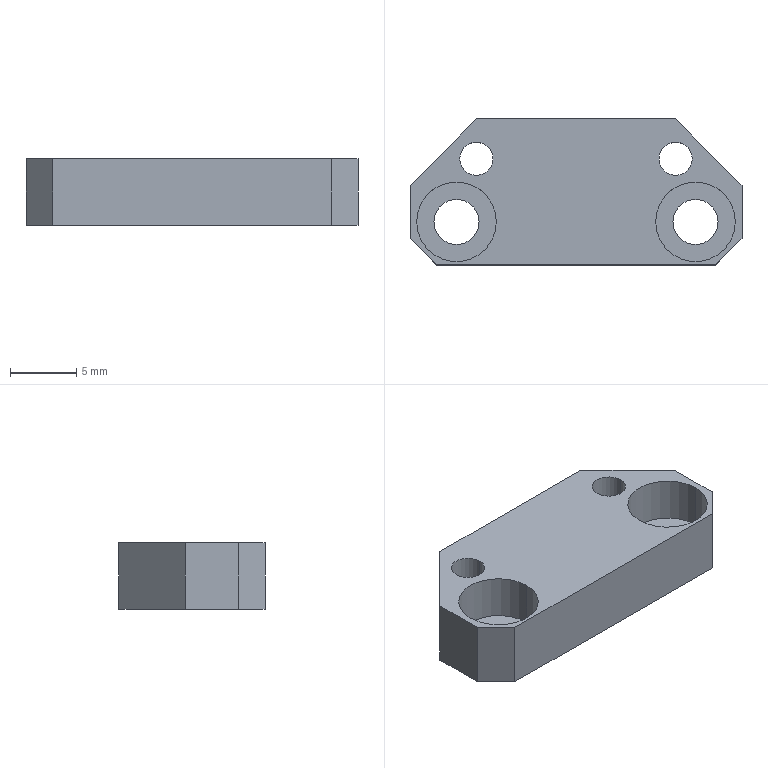Part | SolidWorks | features Chamfer 2, HoleWzd 2, Extrusion 1 | 1 solid | 24 faces | box 25 x 11 x 5 mm | volume 959.594 mm3 | cylinder 12 | plane 12 | commonest cylinder face diameters 2.5 x4 3.4 x4 6 x4
STEP:
#1=CARTESIAN_POINT('',(6.,-2.25,-0.9));
#2=VERTEX_POINT('',#1);
#3=CARTESIAN_POINT('',(12.,-2.25,-0.9));
#4=VERTEX_POINT('',#3);
#5=CARTESIAN_POINT('',(9.,-2.25,-0.9));
#6=DIRECTION('',(0.,0.,1.));
#7=DIRECTION('',(1.,0.,0.));
#8=AXIS2_PLACEMENT_3D('',#5,#6,#7);
#9=CIRCLE('',#8,3.);
#10=EDGE_CURVE('',#2,#4,#9,.T.);
#11=ORIENTED_EDGE('',*,*,#10,.F.);
#12=CARTESIAN_POINT('',(6.,-2.25,2.5));
#13=VERTEX_POINT('',#12);
#14=CARTESIAN_POINT('',(6.,-2.25,2.5));
#15=DIRECTION('',(0.,0.,1.));
#16=VECTOR('',#15,1000.);
#17=LINE('',#14,#16);
#18=EDGE_CURVE('',#2,#13,#17,.T.);
#19=ORIENTED_EDGE('',*,*,#18,.T.);
#20=CARTESIAN_POINT('',(12.,-2.25,2.5));
#21=VERTEX_POINT('',#20);
#22=CARTESIAN_POINT('',(9.,-2.25,2.5));
#23=DIRECTION('',(0.,0.,1.));
#24=DIRECTION('',(1.,0.,0.));
#25=AXIS2_PLACEMENT_3D('',#22,#23,#24);
#26=CIRCLE('',#25,3.);
#27=EDGE_CURVE('',#13,#21,#26,.T.);
#28=ORIENTED_EDGE('',*,*,#27,.T.);
#29=CARTESIAN_POINT('',(12.,-2.25,2.5));
#30=DIRECTION('',(0.,0.,1.));
#31=VECTOR('',#30,1000.);
#32=LINE('',#29,#31);
#33=EDGE_CURVE('',#4,#21,#32,.T.);
#34=ORIENTED_EDGE('',*,*,#33,.F.);
#35=EDGE_LOOP('',(#11,#19,#28,#34));
#36=FACE_OUTER_BOUND('',#35,.T.);
#37=CARTESIAN_POINT('',(9.,-2.25,2.5));
#38=DIRECTION('',(0.,0.,1.));
#39=DIRECTION('',(1.,0.,0.));
#40=AXIS2_PLACEMENT_3D('',#37,#38,#39);
#41=CYLINDRICAL_SURFACE('',#40,3.);
#42=ADVANCED_FACE('',(#36),#41,.F.);
#43=CARTESIAN_POINT('',(7.3,-2.25,-2.5));
#44=VERTEX_POINT('',#43);
#45=CARTESIAN_POINT('',(10.7,-2.25,-2.5));
#46=VERTEX_POINT('',#45);
#47=CARTESIAN_POINT('',(9.,-2.25,-2.5));
#48=DIRECTION('',(0.,0.,1.));
#49=DIRECTION('',(1.,0.,0.));
#50=AXIS2_PLACEMENT_3D('',#47,#48,#49);
#51=CIRCLE('',#50,1.7);
#52=EDGE_CURVE('',#44,#46,#51,.T.);
#53=ORIENTED_EDGE('',*,*,#52,.F.);
#54=CARTESIAN_POINT('',(7.3,-2.25,-0.9));
#55=VERTEX_POINT('',#54);
#56=CARTESIAN_POINT('',(7.3,-2.25,2.5));
#57=DIRECTION('',(0.,0.,1.));
#58=VECTOR('',#57,1000.);
#59=LINE('',#56,#58);
#60=EDGE_CURVE('',#44,#55,#59,.T.);
#61=ORIENTED_EDGE('',*,*,#60,.T.);
#62=CARTESIAN_POINT('',(10.7,-2.25,-0.9));
#63=VERTEX_POINT('',#62);
#64=CARTESIAN_POINT('',(9.,-2.25,-0.9));
#65=DIRECTION('',(0.,0.,1.));
#66=DIRECTION('',(1.,0.,0.));
#67=AXIS2_PLACEMENT_3D('',#64,#65,#66);
#68=CIRCLE('',#67,1.7);
#69=EDGE_CURVE('',#55,#63,#68,.T.);
#70=ORIENTED_EDGE('',*,*,#69,.T.);
#71=CARTESIAN_POINT('',(10.7,-2.25,2.5));
#72=DIRECTION('',(0.,0.,1.));
#73=VECTOR('',#72,1000.);
#74=LINE('',#71,#73);
#75=EDGE_CURVE('',#46,#63,#74,.T.);
#76=ORIENTED_EDGE('',*,*,#75,.F.);
#77=EDGE_LOOP('',(#53,#61,#70,#76));
#78=FACE_OUTER_BOUND('',#77,.T.);
#79=CARTESIAN_POINT('',(9.,-2.25,2.5));
#80=DIRECTION('',(0.,0.,1.));
#81=DIRECTION('',(1.,0.,0.));
#82=AXIS2_PLACEMENT_3D('',#79,#80,#81);
#83=CYLINDRICAL_SURFACE('',#82,1.7);
#84=ADVANCED_FACE('',(#78),#83,.F.);
#85=CARTESIAN_POINT('',(-12.,-2.25,-0.9));
#86=VERTEX_POINT('',#85);
#87=CARTESIAN_POINT('',(-6.,-2.25,-0.9));
#88=VERTEX_POINT('',#87);
#89=CARTESIAN_POINT('',(-9.,-2.25,-0.9));
#90=DIRECTION('',(0.,0.,1.));
#91=DIRECTION('',(1.,0.,0.));
#92=AXIS2_PLACEMENT_3D('',#89,#90,#91);
#93=CIRCLE('',#92,3.);
#94=EDGE_CURVE('',#86,#88,#93,.T.);
#95=ORIENTED_EDGE('',*,*,#94,.F.);
#96=CARTESIAN_POINT('',(-12.,-2.25,2.5));
#97=VERTEX_POINT('',#96);
#98=CARTESIAN_POINT('',(-12.,-2.25,2.5));
#99=DIRECTION('',(0.,0.,1.));
#100=VECTOR('',#99,1000.);
#101=LINE('',#98,#100);
#102=EDGE_CURVE('',#86,#97,#101,.T.);
#103=ORIENTED_EDGE('',*,*,#102,.T.);
#104=CARTESIAN_POINT('',(-6.,-2.25,2.5));
#105=VERTEX_POINT('',#104);
#106=CARTESIAN_POINT('',(-9.,-2.25,2.5));
#107=DIRECTION('',(0.,0.,1.));
#108=DIRECTION('',(1.,0.,0.));
#109=AXIS2_PLACEMENT_3D('',#106,#107,#108);
#110=CIRCLE('',#109,3.);
#111=EDGE_CURVE('',#97,#105,#110,.T.);
#112=ORIENTED_EDGE('',*,*,#111,.T.);
#113=CARTESIAN_POINT('',(-6.,-2.25,2.5));
#114=DIRECTION('',(0.,0.,1.));
#115=VECTOR('',#114,1000.);
#116=LINE('',#113,#115);
#117=EDGE_CURVE('',#88,#105,#116,.T.);
#118=ORIENTED_EDGE('',*,*,#117,.F.);
#119=EDGE_LOOP('',(#95,#103,#112,#118));
#120=FACE_OUTER_BOUND('',#119,.T.);
#121=CARTESIAN_POINT('',(-9.,-2.25,2.5));
#122=DIRECTION('',(0.,0.,1.));
#123=DIRECTION('',(1.,0.,0.));
#124=AXIS2_PLACEMENT_3D('',#121,#122,#123);
#125=CYLINDRICAL_SURFACE('',#124,3.);
#126=ADVANCED_FACE('',(#120),#125,.F.);
#127=CARTESIAN_POINT('',(-10.7,-2.25,-2.5));
#128=VERTEX_POINT('',#127);
#129=CARTESIAN_POINT('',(-7.3,-2.25,-2.5));
#130=VERTEX_POINT('',#129);
#131=CARTESIAN_POINT('',(-9.,-2.25,-2.5));
#132=DIRECTION('',(0.,0.,1.));
#133=DIRECTION('',(1.,0.,0.));
#134=AXIS2_PLACEMENT_3D('',#131,#132,#133);
#135=CIRCLE('',#134,1.7);
#136=EDGE_CURVE('',#128,#130,#135,.T.);
#137=ORIENTED_EDGE('',*,*,#136,.F.);
#138=CARTESIAN_POINT('',(-10.7,-2.25,-0.9));
#139=VERTEX_POINT('',#138);
#140=CARTESIAN_POINT('',(-10.7,-2.25,2.5));
#141=DIRECTION('',(0.,0.,1.));
#142=VECTOR('',#141,1000.);
#143=LINE('',#140,#142);
#144=EDGE_CURVE('',#128,#139,#143,.T.);
#145=ORIENTED_EDGE('',*,*,#144,.T.);
#146=CARTESIAN_POINT('',(-7.3,-2.25,-0.9));
#147=VERTEX_POINT('',#146);
#148=CARTESIAN_POINT('',(-9.,-2.25,-0.9));
#149=DIRECTION('',(0.,0.,1.));
#150=DIRECTION('',(1.,0.,0.));
#151=AXIS2_PLACEMENT_3D('',#148,#149,#150);
#152=CIRCLE('',#151,1.7);
#153=EDGE_CURVE('',#139,#147,#152,.T.);
#154=ORIENTED_EDGE('',*,*,#153,.T.);
#155=CARTESIAN_POINT('',(-7.3,-2.25,2.5));
#156=DIRECTION('',(0.,0.,1.));
#157=VECTOR('',#156,1000.);
#158=LINE('',#155,#157);
#159=EDGE_CURVE('',#130,#147,#158,.T.);
#160=ORIENTED_EDGE('',*,*,#159,.F.);
#161=EDGE_LOOP('',(#137,#145,#154,#160));
#162=FACE_OUTER_BOUND('',#161,.T.);
#163=CARTESIAN_POINT('',(-9.,-2.25,2.5));
#164=DIRECTION('',(0.,0.,1.));
#165=DIRECTION('',(1.,0.,0.));
#166=AXIS2_PLACEMENT_3D('',#163,#164,#165);
#167=CYLINDRICAL_SURFACE('',#166,1.7);
#168=ADVANCED_FACE('',(#162),#167,.F.);
#169=CARTESIAN_POINT('',(-8.75,2.5,-2.5));
#170=VERTEX_POINT('',#169);
#171=CARTESIAN_POINT('',(-6.25,2.5,-2.5));
#172=VERTEX_POINT('',#171);
#173=CARTESIAN_POINT('',(-7.5,2.5,-2.5));
#174=DIRECTION('',(0.,0.,1.));
#175=DIRECTION('',(1.,0.,0.));
#176=AXIS2_PLACEMENT_3D('',#173,#174,#175);
#177=CIRCLE('',#176,1.25);
#178=EDGE_CURVE('',#170,#172,#177,.T.);
#179=ORIENTED_EDGE('',*,*,#178,.F.);
#180=CARTESIAN_POINT('',(-8.75,2.5,2.5));
#181=VERTEX_POINT('',#180);
#182=CARTESIAN_POINT('',(-8.75,2.5,2.5));
#183=DIRECTION('',(0.,0.,1.));
#184=VECTOR('',#183,1000.);
#185=LINE('',#182,#184);
#186=EDGE_CURVE('',#170,#181,#185,.T.);
#187=ORIENTED_EDGE('',*,*,#186,.T.);
#188=CARTESIAN_POINT('',(-6.25,2.5,2.5));
#189=VERTEX_POINT('',#188);
#190=CARTESIAN_POINT('',(-7.5,2.5,2.5));
#191=DIRECTION('',(0.,0.,1.));
#192=DIRECTION('',(1.,0.,0.));
#193=AXIS2_PLACEMENT_3D('',#190,#191,#192);
#194=CIRCLE('',#193,1.25);
#195=EDGE_CURVE('',#181,#189,#194,.T.);
#196=ORIENTED_EDGE('',*,*,#195,.T.);
#197=CARTESIAN_POINT('',(-6.25,2.5,2.5));
#198=DIRECTION('',(0.,0.,1.));
#199=VECTOR('',#198,1000.);
#200=LINE('',#197,#199);
#201=EDGE_CURVE('',#172,#189,#200,.T.);
#202=ORIENTED_EDGE('',*,*,#201,.F.);
#203=EDGE_LOOP('',(#179,#187,#196,#202));
#204=FACE_OUTER_BOUND('',#203,.T.);
#205=CARTESIAN_POINT('',(-7.5,2.5,2.5));
#206=DIRECTION('',(0.,0.,1.));
#207=DIRECTION('',(1.,0.,0.));
#208=AXIS2_PLACEMENT_3D('',#205,#206,#207);
#209=CYLINDRICAL_SURFACE('',#208,1.25);
#210=ADVANCED_FACE('',(#204),#209,.F.);
#211=CARTESIAN_POINT('',(6.25,2.5,-2.5));
#212=VERTEX_POINT('',#211);
#213=CARTESIAN_POINT('',(8.75,2.5,-2.5));
#214=VERTEX_POINT('',#213);
#215=CARTESIAN_POINT('',(7.5,2.5,-2.5));
#216=DIRECTION('',(0.,0.,1.));
#217=DIRECTION('',(1.,0.,0.));
#218=AXIS2_PLACEMENT_3D('',#215,#216,#217);
#219=CIRCLE('',#218,1.25);
#220=EDGE_CURVE('',#212,#214,#219,.T.);
#221=ORIENTED_EDGE('',*,*,#220,.F.);
#222=CARTESIAN_POINT('',(6.25,2.5,2.5));
#223=VERTEX_POINT('',#222);
#224=CARTESIAN_POINT('',(6.25,2.5,2.5));
#225=DIRECTION('',(0.,0.,1.));
#226=VECTOR('',#225,1000.);
#227=LINE('',#224,#226);
#228=EDGE_CURVE('',#212,#223,#227,.T.);
#229=ORIENTED_EDGE('',*,*,#228,.T.);
#230=CARTESIAN_POINT('',(8.75,2.5,2.5));
#231=VERTEX_POINT('',#230);
#232=CARTESIAN_POINT('',(7.5,2.5,2.5));
#233=DIRECTION('',(0.,0.,1.));
#234=DIRECTION('',(1.,0.,0.));
#235=AXIS2_PLACEMENT_3D('',#232,#233,#234);
#236=CIRCLE('',#235,1.25);
#237=EDGE_CURVE('',#223,#231,#236,.T.);
#238=ORIENTED_EDGE('',*,*,#237,.T.);
#239=CARTESIAN_POINT('',(8.75,2.5,2.5));
#240=DIRECTION('',(0.,0.,1.));
#241=VECTOR('',#240,1000.);
#242=LINE('',#239,#241);
#243=EDGE_CURVE('',#214,#231,#242,.T.);
#244=ORIENTED_EDGE('',*,*,#243,.F.);
#245=EDGE_LOOP('',(#221,#229,#238,#244));
#246=FACE_OUTER_BOUND('',#245,.T.);
#247=CARTESIAN_POINT('',(7.5,2.5,2.5));
#248=DIRECTION('',(0.,0.,1.));
#249=DIRECTION('',(1.,0.,0.));
#250=AXIS2_PLACEMENT_3D('',#247,#248,#249);
#251=CYLINDRICAL_SURFACE('',#250,1.25);
#252=ADVANCED_FACE('',(#246),#251,.F.);
#253=CARTESIAN_POINT('',(-7.5,5.5,-2.5));
#254=VERTEX_POINT('',#253);
#255=CARTESIAN_POINT('',(7.5,5.5,-2.5));
#256=VERTEX_POINT('',#255);
#257=CARTESIAN_POINT('',(0.,5.5,-2.5));
#258=DIRECTION('',(1.,0.,0.));
#259=VECTOR('',#258,1000.);
#260=LINE('',#257,#259);
#261=EDGE_CURVE('',#254,#256,#260,.T.);
#262=ORIENTED_EDGE('',*,*,#261,.F.);
#263=CARTESIAN_POINT('',(-7.5,5.5,2.5));
#264=VERTEX_POINT('',#263);
#265=CARTESIAN_POINT('',(-7.5,5.5,2.5));
#266=DIRECTION('',(0.,0.,1.));
#267=VECTOR('',#266,1000.);
#268=LINE('',#265,#267);
#269=EDGE_CURVE('',#254,#264,#268,.T.);
#270=ORIENTED_EDGE('',*,*,#269,.T.);
#271=CARTESIAN_POINT('',(7.5,5.5,2.5));
#272=VERTEX_POINT('',#271);
#273=CARTESIAN_POINT('',(0.,5.5,2.5));
#274=DIRECTION('',(1.,0.,0.));
#275=VECTOR('',#274,1000.);
#276=LINE('',#273,#275);
#277=EDGE_CURVE('',#264,#272,#276,.T.);
#278=ORIENTED_EDGE('',*,*,#277,.T.);
#279=CARTESIAN_POINT('',(7.5,5.5,-2.5));
#280=DIRECTION('',(0.,0.,-1.));
#281=VECTOR('',#280,1000.);
#282=LINE('',#279,#281);
#283=EDGE_CURVE('',#272,#256,#282,.T.);
#284=ORIENTED_EDGE('',*,*,#283,.T.);
#285=EDGE_LOOP('',(#262,#270,#278,#284));
#286=FACE_OUTER_BOUND('',#285,.T.);
#287=CARTESIAN_POINT('',(0.,5.5,2.5));
#288=DIRECTION('',(0.,1.,0.));
#289=DIRECTION('',(0.,0.,1.));
#290=AXIS2_PLACEMENT_3D('',#287,#288,#289);
#291=PLANE('',#290);
#292=ADVANCED_FACE('',(#286),#291,.T.);
#293=CARTESIAN_POINT('',(-12.5,-3.5,-2.5));
#294=VERTEX_POINT('',#293);
#295=CARTESIAN_POINT('',(-12.5,0.5,-2.5));
#296=VERTEX_POINT('',#295);
#297=CARTESIAN_POINT('',(-12.5,0.,-2.5));
#298=DIRECTION('',(0.,1.,0.));
#299=VECTOR('',#298,1000.);
#300=LINE('',#297,#299);
#301=EDGE_CURVE('',#294,#296,#300,.T.);
#302=ORIENTED_EDGE('',*,*,#301,.F.);
#303=CARTESIAN_POINT('',(-12.5,-3.5,2.5));
#304=VERTEX_POINT('',#303);
#305=CARTESIAN_POINT('',(-12.5,-3.5,2.5));
#306=DIRECTION('',(0.,0.,1.));
#307=VECTOR('',#306,1000.);
#308=LINE('',#305,#307);
#309=EDGE_CURVE('',#294,#304,#308,.T.);
#310=ORIENTED_EDGE('',*,*,#309,.T.);
#311=CARTESIAN_POINT('',(-12.5,0.5,2.5));
#312=VERTEX_POINT('',#311);
#313=CARTESIAN_POINT('',(-12.5,0.,2.5));
#314=DIRECTION('',(0.,1.,0.));
#315=VECTOR('',#314,1000.);
#316=LINE('',#313,#315);
#317=EDGE_CURVE('',#304,#312,#316,.T.);
#318=ORIENTED_EDGE('',*,*,#317,.T.);
#319=CARTESIAN_POINT('',(-12.5,0.5,2.5));
#320=DIRECTION('',(0.,0.,-1.));
#321=VECTOR('',#320,1000.);
#322=LINE('',#319,#321);
#323=EDGE_CURVE('',#312,#296,#322,.T.);
#324=ORIENTED_EDGE('',*,*,#323,.T.);
#325=EDGE_LOOP('',(#302,#310,#318,#324));
#326=FACE_OUTER_BOUND('',#325,.T.);
#327=CARTESIAN_POINT('',(-12.5,0.,2.5));
#328=DIRECTION('',(-1.,0.,0.));
#329=DIRECTION('',(0.,0.,1.));
#330=AXIS2_PLACEMENT_3D('',#327,#328,#329);
#331=PLANE('',#330);
#332=ADVANCED_FACE('',(#326),#331,.T.);
#333=CARTESIAN_POINT('',(-10.5,-5.5,2.5));
#334=VERTEX_POINT('',#333);
#335=CARTESIAN_POINT('',(10.5,-5.5,2.5));
#336=VERTEX_POINT('',#335);
#337=CARTESIAN_POINT('',(0.,-5.5,2.5));
#338=DIRECTION('',(1.,0.,0.));
#339=VECTOR('',#338,1000.);
#340=LINE('',#337,#339);
#341=EDGE_CURVE('',#334,#336,#340,.T.);
#342=ORIENTED_EDGE('',*,*,#341,.F.);
#343=CARTESIAN_POINT('',(-10.5,-5.5,-2.5));
#344=VERTEX_POINT('',#343);
#345=CARTESIAN_POINT('',(-10.5,-5.5,-2.5));
#346=DIRECTION('',(0.,0.,-1.));
#347=VECTOR('',#346,1000.);
#348=LINE('',#345,#347);
#349=EDGE_CURVE('',#334,#344,#348,.T.);
#350=ORIENTED_EDGE('',*,*,#349,.T.);
#351=CARTESIAN_POINT('',(10.5,-5.5,-2.5));
#352=VERTEX_POINT('',#351);
#353=CARTESIAN_POINT('',(0.,-5.5,-2.5));
#354=DIRECTION('',(1.,0.,0.));
#355=VECTOR('',#354,1000.);
#356=LINE('',#353,#355);
#357=EDGE_CURVE('',#344,#352,#356,.T.);
#358=ORIENTED_EDGE('',*,*,#357,.T.);
#359=CARTESIAN_POINT('',(10.5,-5.5,2.5));
#360=DIRECTION('',(0.,0.,1.));
#361=VECTOR('',#360,1000.);
#362=LINE('',#359,#361);
#363=EDGE_CURVE('',#352,#336,#362,.T.);
#364=ORIENTED_EDGE('',*,*,#363,.T.);
#365=EDGE_LOOP('',(#342,#350,#358,#364));
#366=FACE_OUTER_BOUND('',#365,.T.);
#367=CARTESIAN_POINT('',(0.,-5.5,2.5));
#368=DIRECTION('',(0.,1.,0.));
#369=DIRECTION('',(-1.,0.,0.));
#370=AXIS2_PLACEMENT_3D('',#367,#368,#369);
#371=PLANE('',#370);
#372=ADVANCED_FACE('',(#366),#371,.F.);
#373=CARTESIAN_POINT('',(12.5,-3.5,2.5));
#374=VERTEX_POINT('',#373);
#375=CARTESIAN_POINT('',(12.5,0.5,2.5));
#376=VERTEX_POINT('',#375);
#377=CARTESIAN_POINT('',(12.5,0.,2.5));
#378=DIRECTION('',(0.,1.,0.));
#379=VECTOR('',#378,1000.);
#380=LINE('',#377,#379);
#381=EDGE_CURVE('',#374,#376,#380,.T.);
#382=ORIENTED_EDGE('',*,*,#381,.F.);
#383=CARTESIAN_POINT('',(12.5,-3.5,-2.5));
#384=VERTEX_POINT('',#383);
#385=CARTESIAN_POINT('',(12.5,-3.5,2.5));
#386=DIRECTION('',(0.,0.,-1.));
#387=VECTOR('',#386,1000.);
#388=LINE('',#385,#387);
#389=EDGE_CURVE('',#374,#384,#388,.T.);
#390=ORIENTED_EDGE('',*,*,#389,.T.);
#391=CARTESIAN_POINT('',(12.5,0.5,-2.5));
#392=VERTEX_POINT('',#391);
#393=CARTESIAN_POINT('',(12.5,0.,-2.5));
#394=DIRECTION('',(0.,1.,0.));
#395=VECTOR('',#394,1000.);
#396=LINE('',#393,#395);
#397=EDGE_CURVE('',#384,#392,#396,.T.);
#398=ORIENTED_EDGE('',*,*,#397,.T.);
#399=CARTESIAN_POINT('',(12.5,0.5,2.5));
#400=DIRECTION('',(0.,0.,1.));
#401=VECTOR('',#400,1000.);
#402=LINE('',#399,#401);
#403=EDGE_CURVE('',#392,#376,#402,.T.);
#404=ORIENTED_EDGE('',*,*,#403,.T.);
#405=EDGE_LOOP('',(#382,#390,#398,#404));
#406=FACE_OUTER_BOUND('',#405,.T.);
#407=CARTESIAN_POINT('',(12.5,0.,2.5));
#408=DIRECTION('',(-1.,0.,0.));
#409=DIRECTION('',(0.,0.,1.));
#410=AXIS2_PLACEMENT_3D('',#407,#408,#409);
#411=PLANE('',#410);
#412=ADVANCED_FACE('',(#406),#411,.F.);
#413=CARTESIAN_POINT('',(9.,-2.25,2.5));
#414=DIRECTION('',(0.,0.,1.));
#415=DIRECTION('',(1.,0.,0.));
#416=AXIS2_PLACEMENT_3D('',#413,#414,#415);
#417=CIRCLE('',#416,3.);
#418=EDGE_CURVE('',#21,#13,#417,.T.);
#419=ORIENTED_EDGE('',*,*,#418,.F.);
#420=ORIENTED_EDGE('',*,*,#27,.F.);
#421=EDGE_LOOP('',(#419,#420));
#422=FACE_BOUND('',#421,.T.);
#423=CARTESIAN_POINT('',(-9.,-2.25,2.5));
#424=DIRECTION('',(0.,0.,1.));
#425=DIRECTION('',(1.,0.,0.));
#426=AXIS2_PLACEMENT_3D('',#423,#424,#425);
#427=CIRCLE('',#426,3.);
#428=EDGE_CURVE('',#105,#97,#427,.T.);
#429=ORIENTED_EDGE('',*,*,#428,.F.);
#430=ORIENTED_EDGE('',*,*,#111,.F.);
#431=EDGE_LOOP('',(#429,#430));
#432=FACE_BOUND('',#431,.T.);
#433=CARTESIAN_POINT('',(-7.5,2.5,2.5));
#434=DIRECTION('',(0.,0.,1.));
#435=DIRECTION('',(1.,0.,0.));
#436=AXIS2_PLACEMENT_3D('',#433,#434,#435);
#437=CIRCLE('',#436,1.25);
#438=EDGE_CURVE('',#189,#181,#437,.T.);
#439=ORIENTED_EDGE('',*,*,#438,.F.);
#440=ORIENTED_EDGE('',*,*,#195,.F.);
#441=EDGE_LOOP('',(#439,#440));
#442=FACE_BOUND('',#441,.T.);
#443=CARTESIAN_POINT('',(7.5,2.5,2.5));
#444=DIRECTION('',(0.,0.,1.));
#445=DIRECTION('',(1.,0.,0.));
#446=AXIS2_PLACEMENT_3D('',#443,#444,#445);
#447=CIRCLE('',#446,1.25);
#448=EDGE_CURVE('',#231,#223,#447,.T.);
#449=ORIENTED_EDGE('',*,*,#448,.F.);
#450=ORIENTED_EDGE('',*,*,#237,.F.);
#451=EDGE_LOOP('',(#449,#450));
#452=FACE_BOUND('',#451,.T.);
#453=ORIENTED_EDGE('',*,*,#317,.F.);
#454=CARTESIAN_POINT('',(-8.,-8.,2.5));
#455=DIRECTION('',(0.7071,-0.7071,0.));
#456=VECTOR('',#455,1000.);
#457=LINE('',#454,#456);
#458=EDGE_CURVE('',#304,#334,#457,.T.);
#459=ORIENTED_EDGE('',*,*,#458,.T.);
#460=ORIENTED_EDGE('',*,*,#341,.T.);
#461=CARTESIAN_POINT('',(8.,-8.,2.5));
#462=DIRECTION('',(0.7071,0.7071,0.));
#463=VECTOR('',#462,1000.);
#464=LINE('',#461,#463);
#465=EDGE_CURVE('',#336,#374,#464,.T.);
#466=ORIENTED_EDGE('',*,*,#465,.T.);
#467=ORIENTED_EDGE('',*,*,#381,.T.);
#468=CARTESIAN_POINT('',(6.5,6.5,2.5));
#469=DIRECTION('',(-0.7071,0.7071,0.));
#470=VECTOR('',#469,1000.);
#471=LINE('',#468,#470);
#472=EDGE_CURVE('',#376,#272,#471,.T.);
#473=ORIENTED_EDGE('',*,*,#472,.T.);
#474=ORIENTED_EDGE('',*,*,#277,.F.);
#475=CARTESIAN_POINT('',(-6.5,6.5,2.5));
#476=DIRECTION('',(-0.7071,-0.7071,0.));
#477=VECTOR('',#476,1000.);
#478=LINE('',#475,#477);
#479=EDGE_CURVE('',#264,#312,#478,.T.);
#480=ORIENTED_EDGE('',*,*,#479,.T.);
#481=EDGE_LOOP('',(#453,#459,#460,#466,#467,#473,#474,#480));
#482=FACE_OUTER_BOUND('',#481,.T.);
#483=CARTESIAN_POINT('',(0.,0.,2.5));
#484=DIRECTION('',(0.,0.,1.));
#485=DIRECTION('',(1.,0.,0.));
#486=AXIS2_PLACEMENT_3D('',#483,#484,#485);
#487=PLANE('',#486);
#488=ADVANCED_FACE('',(#422,#432,#442,#452,#482),#487,.T.);
#489=CARTESIAN_POINT('',(9.,-2.25,-2.5));
#490=DIRECTION('',(0.,0.,1.));
#491=DIRECTION('',(1.,0.,0.));
#492=AXIS2_PLACEMENT_3D('',#489,#490,#491);
#493=CIRCLE('',#492,1.7);
#494=EDGE_CURVE('',#46,#44,#493,.T.);
#495=ORIENTED_EDGE('',*,*,#494,.T.);
#496=ORIENTED_EDGE('',*,*,#52,.T.);
#497=EDGE_LOOP('',(#495,#496));
#498=FACE_BOUND('',#497,.T.);
#499=CARTESIAN_POINT('',(-9.,-2.25,-2.5));
#500=DIRECTION('',(0.,0.,1.));
#501=DIRECTION('',(1.,0.,0.));
#502=AXIS2_PLACEMENT_3D('',#499,#500,#501);
#503=CIRCLE('',#502,1.7);
#504=EDGE_CURVE('',#130,#128,#503,.T.);
#505=ORIENTED_EDGE('',*,*,#504,.T.);
#506=ORIENTED_EDGE('',*,*,#136,.T.);
#507=EDGE_LOOP('',(#505,#506));
#508=FACE_BOUND('',#507,.T.);
#509=CARTESIAN_POINT('',(-7.5,2.5,-2.5));
#510=DIRECTION('',(0.,0.,1.));
#511=DIRECTION('',(1.,0.,0.));
#512=AXIS2_PLACEMENT_3D('',#509,#510,#511);
#513=CIRCLE('',#512,1.25);
#514=EDGE_CURVE('',#172,#170,#513,.T.);
#515=ORIENTED_EDGE('',*,*,#514,.T.);
#516=ORIENTED_EDGE('',*,*,#178,.T.);
#517=EDGE_LOOP('',(#515,#516));
#518=FACE_BOUND('',#517,.T.);
#519=CARTESIAN_POINT('',(7.5,2.5,-2.5));
#520=DIRECTION('',(0.,0.,1.));
#521=DIRECTION('',(1.,0.,0.));
#522=AXIS2_PLACEMENT_3D('',#519,#520,#521);
#523=CIRCLE('',#522,1.25);
#524=EDGE_CURVE('',#214,#212,#523,.T.);
#525=ORIENTED_EDGE('',*,*,#524,.T.);
#526=ORIENTED_EDGE('',*,*,#220,.T.);
#527=EDGE_LOOP('',(#525,#526));
#528=FACE_BOUND('',#527,.T.);
#529=ORIENTED_EDGE('',*,*,#357,.F.);
#530=CARTESIAN_POINT('',(-10.5,-5.5,-2.5));
#531=DIRECTION('',(-0.7071,0.7071,0.));
#532=VECTOR('',#531,1000.);
#533=LINE('',#530,#532);
#534=EDGE_CURVE('',#344,#294,#533,.T.);
#535=ORIENTED_EDGE('',*,*,#534,.T.);
#536=ORIENTED_EDGE('',*,*,#301,.T.);
#537=CARTESIAN_POINT('',(-12.5,0.5,-2.5));
#538=DIRECTION('',(0.7071,0.7071,0.));
#539=VECTOR('',#538,1000.);
#540=LINE('',#537,#539);
#541=EDGE_CURVE('',#296,#254,#540,.T.);
#542=ORIENTED_EDGE('',*,*,#541,.T.);
#543=ORIENTED_EDGE('',*,*,#261,.T.);
#544=CARTESIAN_POINT('',(7.5,5.5,-2.5));
#545=DIRECTION('',(0.7071,-0.7071,0.));
#546=VECTOR('',#545,1000.);
#547=LINE('',#544,#546);
#548=EDGE_CURVE('',#256,#392,#547,.T.);
#549=ORIENTED_EDGE('',*,*,#548,.T.);
#550=ORIENTED_EDGE('',*,*,#397,.F.);
#551=CARTESIAN_POINT('',(12.5,-3.5,-2.5));
#552=DIRECTION('',(-0.7071,-0.7071,0.));
#553=VECTOR('',#552,1000.);
#554=LINE('',#551,#553);
#555=EDGE_CURVE('',#384,#352,#554,.T.);
#556=ORIENTED_EDGE('',*,*,#555,.T.);
#557=EDGE_LOOP('',(#529,#535,#536,#542,#543,#549,#550,#556));
#558=FACE_OUTER_BOUND('',#557,.T.);
#559=CARTESIAN_POINT('',(0.,0.,-2.5));
#560=DIRECTION('',(0.,0.,1.));
#561=DIRECTION('',(1.,0.,0.));
#562=AXIS2_PLACEMENT_3D('',#559,#560,#561);
#563=PLANE('',#562);
#564=ADVANCED_FACE('',(#498,#508,#518,#528,#558),#563,.F.);
#565=ORIENTED_EDGE('',*,*,#228,.F.);
#566=ORIENTED_EDGE('',*,*,#524,.F.);
#567=ORIENTED_EDGE('',*,*,#243,.T.);
#568=ORIENTED_EDGE('',*,*,#448,.T.);
#569=EDGE_LOOP('',(#565,#566,#567,#568));
#570=FACE_OUTER_BOUND('',#569,.T.);
#571=CARTESIAN_POINT('',(7.5,2.5,2.5));
#572=DIRECTION('',(0.,0.,1.));
#573=DIRECTION('',(1.,0.,0.));
#574=AXIS2_PLACEMENT_3D('',#571,#572,#573);
#575=CYLINDRICAL_SURFACE('',#574,1.25);
#576=ADVANCED_FACE('',(#570),#575,.F.);
#577=ORIENTED_EDGE('',*,*,#186,.F.);
#578=ORIENTED_EDGE('',*,*,#514,.F.);
#579=ORIENTED_EDGE('',*,*,#201,.T.);
#580=ORIENTED_EDGE('',*,*,#438,.T.);
#581=EDGE_LOOP('',(#577,#578,#579,#580));
#582=FACE_OUTER_BOUND('',#581,.T.);
#583=CARTESIAN_POINT('',(-7.5,2.5,2.5));
#584=DIRECTION('',(0.,0.,1.));
#585=DIRECTION('',(1.,0.,0.));
#586=AXIS2_PLACEMENT_3D('',#583,#584,#585);
#587=CYLINDRICAL_SURFACE('',#586,1.25);
#588=ADVANCED_FACE('',(#582),#587,.F.);
#589=ORIENTED_EDGE('',*,*,#144,.F.);
#590=ORIENTED_EDGE('',*,*,#504,.F.);
#591=ORIENTED_EDGE('',*,*,#159,.T.);
#592=CARTESIAN_POINT('',(-9.,-2.25,-0.9));
#593=DIRECTION('',(0.,0.,1.));
#594=DIRECTION('',(1.,0.,0.));
#595=AXIS2_PLACEMENT_3D('',#592,#593,#594);
#596=CIRCLE('',#595,1.7);
#597=EDGE_CURVE('',#147,#139,#596,.T.);
#598=ORIENTED_EDGE('',*,*,#597,.T.);
#599=EDGE_LOOP('',(#589,#590,#591,#598));
#600=FACE_OUTER_BOUND('',#599,.T.);
#601=CARTESIAN_POINT('',(-9.,-2.25,2.5));
#602=DIRECTION('',(0.,0.,1.));
#603=DIRECTION('',(1.,0.,0.));
#604=AXIS2_PLACEMENT_3D('',#601,#602,#603);
#605=CYLINDRICAL_SURFACE('',#604,1.7);
#606=ADVANCED_FACE('',(#600),#605,.F.);
#607=ORIENTED_EDGE('',*,*,#597,.F.);
#608=ORIENTED_EDGE('',*,*,#153,.F.);
#609=EDGE_LOOP('',(#607,#608));
#610=FACE_BOUND('',#609,.T.);
#611=CARTESIAN_POINT('',(-9.,-2.25,-0.9));
#612=DIRECTION('',(0.,0.,1.));
#613=DIRECTION('',(1.,0.,0.));
#614=AXIS2_PLACEMENT_3D('',#611,#612,#613);
#615=CIRCLE('',#614,3.);
#616=EDGE_CURVE('',#88,#86,#615,.T.);
#617=ORIENTED_EDGE('',*,*,#616,.T.);
#618=ORIENTED_EDGE('',*,*,#94,.T.);
#619=EDGE_LOOP('',(#617,#618));
#620=FACE_OUTER_BOUND('',#619,.T.);
#621=CARTESIAN_POINT('',(-7.3,-2.25,-0.9));
#622=DIRECTION('',(0.,0.,-1.));
#623=DIRECTION('',(-1.,0.,0.));
#624=AXIS2_PLACEMENT_3D('',#621,#622,#623);
#625=PLANE('',#624);
#626=ADVANCED_FACE('',(#610,#620),#625,.F.);
#627=ORIENTED_EDGE('',*,*,#102,.F.);
#628=ORIENTED_EDGE('',*,*,#616,.F.);
#629=ORIENTED_EDGE('',*,*,#117,.T.);
#630=ORIENTED_EDGE('',*,*,#428,.T.);
#631=EDGE_LOOP('',(#627,#628,#629,#630));
#632=FACE_OUTER_BOUND('',#631,.T.);
#633=CARTESIAN_POINT('',(-9.,-2.25,2.5));
#634=DIRECTION('',(0.,0.,1.));
#635=DIRECTION('',(1.,0.,0.));
#636=AXIS2_PLACEMENT_3D('',#633,#634,#635);
#637=CYLINDRICAL_SURFACE('',#636,3.);
#638=ADVANCED_FACE('',(#632),#637,.F.);
#639=ORIENTED_EDGE('',*,*,#60,.F.);
#640=ORIENTED_EDGE('',*,*,#494,.F.);
#641=ORIENTED_EDGE('',*,*,#75,.T.);
#642=CARTESIAN_POINT('',(9.,-2.25,-0.9));
#643=DIRECTION('',(0.,0.,1.));
#644=DIRECTION('',(1.,0.,0.));
#645=AXIS2_PLACEMENT_3D('',#642,#643,#644);
#646=CIRCLE('',#645,1.7);
#647=EDGE_CURVE('',#63,#55,#646,.T.);
#648=ORIENTED_EDGE('',*,*,#647,.T.);
#649=EDGE_LOOP('',(#639,#640,#641,#648));
#650=FACE_OUTER_BOUND('',#649,.T.);
#651=CARTESIAN_POINT('',(9.,-2.25,2.5));
#652=DIRECTION('',(0.,0.,1.));
#653=DIRECTION('',(1.,0.,0.));
#654=AXIS2_PLACEMENT_3D('',#651,#652,#653);
#655=CYLINDRICAL_SURFACE('',#654,1.7);
#656=ADVANCED_FACE('',(#650),#655,.F.);
#657=ORIENTED_EDGE('',*,*,#647,.F.);
#658=ORIENTED_EDGE('',*,*,#69,.F.);
#659=EDGE_LOOP('',(#657,#658));
#660=FACE_BOUND('',#659,.T.);
#661=CARTESIAN_POINT('',(9.,-2.25,-0.9));
#662=DIRECTION('',(0.,0.,1.));
#663=DIRECTION('',(1.,0.,0.));
#664=AXIS2_PLACEMENT_3D('',#661,#662,#663);
#665=CIRCLE('',#664,3.);
#666=EDGE_CURVE('',#4,#2,#665,.T.);
#667=ORIENTED_EDGE('',*,*,#666,.T.);
#668=ORIENTED_EDGE('',*,*,#10,.T.);
#669=EDGE_LOOP('',(#667,#668));
#670=FACE_OUTER_BOUND('',#669,.T.);
#671=CARTESIAN_POINT('',(10.7,-2.25,-0.9));
#672=DIRECTION('',(0.,0.,-1.));
#673=DIRECTION('',(-1.,0.,0.));
#674=AXIS2_PLACEMENT_3D('',#671,#672,#673);
#675=PLANE('',#674);
#676=ADVANCED_FACE('',(#660,#670),#675,.F.);
#677=ORIENTED_EDGE('',*,*,#18,.F.);
#678=ORIENTED_EDGE('',*,*,#666,.F.);
#679=ORIENTED_EDGE('',*,*,#33,.T.);
#680=ORIENTED_EDGE('',*,*,#418,.T.);
#681=EDGE_LOOP('',(#677,#678,#679,#680));
#682=FACE_OUTER_BOUND('',#681,.T.);
#683=CARTESIAN_POINT('',(9.,-2.25,2.5));
#684=DIRECTION('',(0.,0.,1.));
#685=DIRECTION('',(1.,0.,0.));
#686=AXIS2_PLACEMENT_3D('',#683,#684,#685);
#687=CYLINDRICAL_SURFACE('',#686,3.);
#688=ADVANCED_FACE('',(#682),#687,.F.);
#689=ORIENTED_EDGE('',*,*,#479,.F.);
#690=ORIENTED_EDGE('',*,*,#269,.F.);
#691=ORIENTED_EDGE('',*,*,#541,.F.);
#692=ORIENTED_EDGE('',*,*,#323,.F.);
#693=EDGE_LOOP('',(#689,#690,#691,#692));
#694=FACE_OUTER_BOUND('',#693,.T.);
#695=CARTESIAN_POINT('',(-12.5,0.5,2.5));
#696=DIRECTION('',(0.7071,-0.7071,0.));
#697=DIRECTION('',(0.,0.,-1.));
#698=AXIS2_PLACEMENT_3D('',#695,#696,#697);
#699=PLANE('',#698);
#700=ADVANCED_FACE('',(#694),#699,.F.);
#701=ORIENTED_EDGE('',*,*,#472,.F.);
#702=ORIENTED_EDGE('',*,*,#403,.F.);
#703=ORIENTED_EDGE('',*,*,#548,.F.);
#704=ORIENTED_EDGE('',*,*,#283,.F.);
#705=EDGE_LOOP('',(#701,#702,#703,#704));
#706=FACE_OUTER_BOUND('',#705,.T.);
#707=CARTESIAN_POINT('',(7.5,5.5,2.5));
#708=DIRECTION('',(0.7071,0.7071,0.));
#709=DIRECTION('',(0.,0.,1.));
#710=AXIS2_PLACEMENT_3D('',#707,#708,#709);
#711=PLANE('',#710);
#712=ADVANCED_FACE('',(#706),#711,.T.);
#713=ORIENTED_EDGE('',*,*,#458,.F.);
#714=ORIENTED_EDGE('',*,*,#309,.F.);
#715=ORIENTED_EDGE('',*,*,#534,.F.);
#716=ORIENTED_EDGE('',*,*,#349,.F.);
#717=EDGE_LOOP('',(#713,#714,#715,#716));
#718=FACE_OUTER_BOUND('',#717,.T.);
#719=CARTESIAN_POINT('',(-10.5,-5.5,2.5));
#720=DIRECTION('',(-0.7071,-0.7071,0.));
#721=DIRECTION('',(0.,0.,1.));
#722=AXIS2_PLACEMENT_3D('',#719,#720,#721);
#723=PLANE('',#722);
#724=ADVANCED_FACE('',(#718),#723,.T.);
#725=ORIENTED_EDGE('',*,*,#465,.F.);
#726=ORIENTED_EDGE('',*,*,#363,.F.);
#727=ORIENTED_EDGE('',*,*,#555,.F.);
#728=ORIENTED_EDGE('',*,*,#389,.F.);
#729=EDGE_LOOP('',(#725,#726,#727,#728));
#730=FACE_OUTER_BOUND('',#729,.T.);
#731=CARTESIAN_POINT('',(12.5,-3.5,2.5));
#732=DIRECTION('',(-0.7071,0.7071,0.));
#733=DIRECTION('',(0.,0.,-1.));
#734=AXIS2_PLACEMENT_3D('',#731,#732,#733);
#735=PLANE('',#734);
#736=ADVANCED_FACE('',(#730),#735,.F.);
#737=CLOSED_SHELL('',(#42,#84,#126,#168,#210,#252,#292,#332,#372,#412,#488,#564,#576,#588,#606,#626,#638,#656,#676,#688,#700,#712,#724,#736));
#738=MANIFOLD_SOLID_BREP('',#737);
#739=CARTESIAN_POINT('',(0.,0.,0.));
#740=DIRECTION('',(0.,0.,1.));
#741=DIRECTION('',(1.,0.,0.));
#742=AXIS2_PLACEMENT_3D('',#739,#740,#741);
#743=(LENGTH_UNIT()NAMED_UNIT(*)SI_UNIT(.MILLI.,.METRE.));
#744=UNCERTAINTY_MEASURE_WITH_UNIT(LENGTH_MEASURE(0.00001),#743,'','');
#745=(NAMED_UNIT(*)PLANE_ANGLE_UNIT()SI_UNIT($,.RADIAN.));
#746=(NAMED_UNIT(*)SI_UNIT($,.STERADIAN.)SOLID_ANGLE_UNIT());
#747=(GEOMETRIC_REPRESENTATION_CONTEXT(3)GLOBAL_UNCERTAINTY_ASSIGNED_CONTEXT((#744))GLOBAL_UNIT_ASSIGNED_CONTEXT((#743,#745,#746))REPRESENTATION_CONTEXT('',''));
#748=ADVANCED_BREP_SHAPE_REPRESENTATION('',(#738,#742),#747);